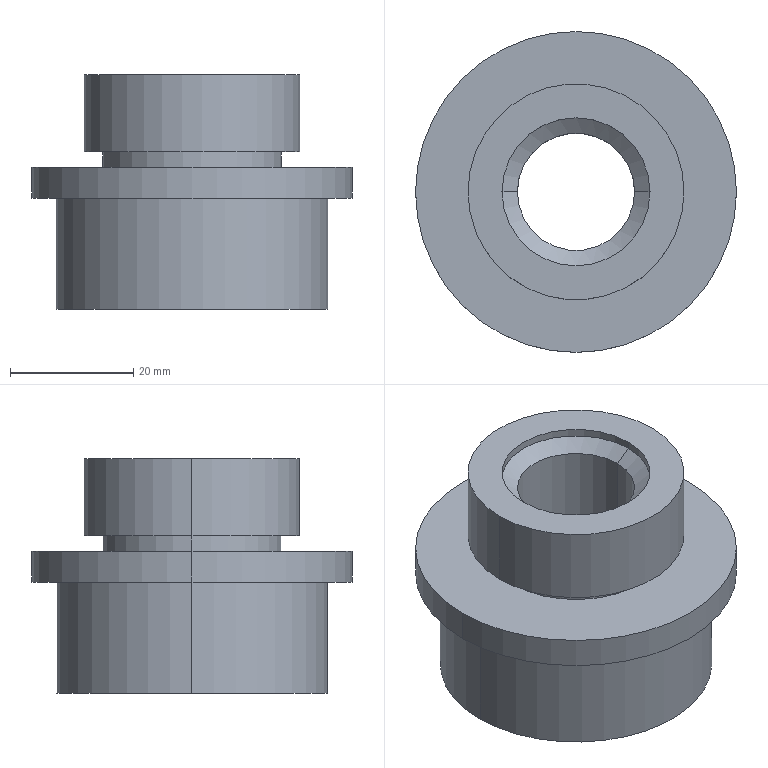Part | SolidWorks | features Revolution 1 | 1 solid | 21 faces | box 52 x 52 x 38 mm | volume 38206 mm3 | cylinder 12 | plane 5 | cone 4 | commonest cylinder face diameters 19 x2 24 x2 29 x2 35 x2 44 x2 52 x2
STEP:
#1=CARTESIAN_POINT('',(17.5,0.,-12.5));
#2=VERTEX_POINT('',#1);
#3=CARTESIAN_POINT('',(-17.5,0.,-12.5));
#4=VERTEX_POINT('',#3);
#5=CARTESIAN_POINT('',(0.,0.,-12.5));
#6=DIRECTION('',(0.,0.,1.));
#7=DIRECTION('',(1.,0.,0.));
#8=AXIS2_PLACEMENT_3D('',#5,#6,#7);
#9=CIRCLE('',#8,17.5);
#10=EDGE_CURVE('',#2,#4,#9,.T.);
#11=ORIENTED_EDGE('',*,*,#10,.T.);
#12=CARTESIAN_POINT('',(-17.5,0.,0.));
#13=VERTEX_POINT('',#12);
#14=CARTESIAN_POINT('',(-17.5,0.,28.492));
#15=DIRECTION('',(0.,0.,1.));
#16=VECTOR('',#15,1000.);
#17=LINE('',#14,#16);
#18=EDGE_CURVE('',#4,#13,#17,.T.);
#19=ORIENTED_EDGE('',*,*,#18,.T.);
#20=CARTESIAN_POINT('',(17.5,0.,0.));
#21=VERTEX_POINT('',#20);
#22=CARTESIAN_POINT('',(0.,0.,0.));
#23=DIRECTION('',(0.,0.,1.));
#24=DIRECTION('',(1.,0.,0.));
#25=AXIS2_PLACEMENT_3D('',#22,#23,#24);
#26=CIRCLE('',#25,17.5);
#27=EDGE_CURVE('',#21,#13,#26,.T.);
#28=ORIENTED_EDGE('',*,*,#27,.F.);
#29=CARTESIAN_POINT('',(17.5,0.,28.492));
#30=DIRECTION('',(0.,0.,1.));
#31=VECTOR('',#30,1000.);
#32=LINE('',#29,#31);
#33=EDGE_CURVE('',#2,#21,#32,.T.);
#34=ORIENTED_EDGE('',*,*,#33,.F.);
#35=EDGE_LOOP('',(#11,#19,#28,#34));
#36=FACE_OUTER_BOUND('',#35,.T.);
#37=CARTESIAN_POINT('',(0.,0.,28.492));
#38=DIRECTION('',(0.,0.,1.));
#39=DIRECTION('',(1.,0.,0.));
#40=AXIS2_PLACEMENT_3D('',#37,#38,#39);
#41=CYLINDRICAL_SURFACE('',#40,17.5);
#42=ADVANCED_FACE('',(#36),#41,.T.);
#43=CARTESIAN_POINT('',(14.5,0.,-15.));
#44=VERTEX_POINT('',#43);
#45=CARTESIAN_POINT('',(-14.5,0.,-15.));
#46=VERTEX_POINT('',#45);
#47=CARTESIAN_POINT('',(0.,0.,-15.));
#48=DIRECTION('',(0.,0.,1.));
#49=DIRECTION('',(1.,0.,0.));
#50=AXIS2_PLACEMENT_3D('',#47,#48,#49);
#51=CIRCLE('',#50,14.5);
#52=EDGE_CURVE('',#44,#46,#51,.T.);
#53=ORIENTED_EDGE('',*,*,#52,.T.);
#54=CARTESIAN_POINT('',(-14.5,0.,-12.5));
#55=VERTEX_POINT('',#54);
#56=CARTESIAN_POINT('',(-14.5,0.,28.492));
#57=DIRECTION('',(0.,0.,1.));
#58=VECTOR('',#57,1000.);
#59=LINE('',#56,#58);
#60=EDGE_CURVE('',#46,#55,#59,.T.);
#61=ORIENTED_EDGE('',*,*,#60,.T.);
#62=CARTESIAN_POINT('',(14.5,0.,-12.5));
#63=VERTEX_POINT('',#62);
#64=CARTESIAN_POINT('',(0.,0.,-12.5));
#65=DIRECTION('',(0.,0.,1.));
#66=DIRECTION('',(1.,0.,0.));
#67=AXIS2_PLACEMENT_3D('',#64,#65,#66);
#68=CIRCLE('',#67,14.5);
#69=EDGE_CURVE('',#63,#55,#68,.T.);
#70=ORIENTED_EDGE('',*,*,#69,.F.);
#71=CARTESIAN_POINT('',(14.5,0.,28.492));
#72=DIRECTION('',(0.,0.,1.));
#73=VECTOR('',#72,1000.);
#74=LINE('',#71,#73);
#75=EDGE_CURVE('',#44,#63,#74,.T.);
#76=ORIENTED_EDGE('',*,*,#75,.F.);
#77=EDGE_LOOP('',(#53,#61,#70,#76));
#78=FACE_OUTER_BOUND('',#77,.T.);
#79=CARTESIAN_POINT('',(0.,0.,28.492));
#80=DIRECTION('',(0.,0.,1.));
#81=DIRECTION('',(1.,0.,0.));
#82=AXIS2_PLACEMENT_3D('',#79,#80,#81);
#83=CYLINDRICAL_SURFACE('',#82,14.5);
#84=ADVANCED_FACE('',(#78),#83,.T.);
#85=CARTESIAN_POINT('',(26.,0.,-20.));
#86=VERTEX_POINT('',#85);
#87=CARTESIAN_POINT('',(-26.,0.,-20.));
#88=VERTEX_POINT('',#87);
#89=CARTESIAN_POINT('',(0.,0.,-20.));
#90=DIRECTION('',(0.,0.,1.));
#91=DIRECTION('',(1.,0.,0.));
#92=AXIS2_PLACEMENT_3D('',#89,#90,#91);
#93=CIRCLE('',#92,26.);
#94=EDGE_CURVE('',#86,#88,#93,.T.);
#95=ORIENTED_EDGE('',*,*,#94,.T.);
#96=CARTESIAN_POINT('',(-26.,0.,-15.));
#97=VERTEX_POINT('',#96);
#98=CARTESIAN_POINT('',(-26.,0.,28.492));
#99=DIRECTION('',(0.,0.,1.));
#100=VECTOR('',#99,1000.);
#101=LINE('',#98,#100);
#102=EDGE_CURVE('',#88,#97,#101,.T.);
#103=ORIENTED_EDGE('',*,*,#102,.T.);
#104=CARTESIAN_POINT('',(26.,0.,-15.));
#105=VERTEX_POINT('',#104);
#106=CARTESIAN_POINT('',(0.,0.,-15.));
#107=DIRECTION('',(0.,0.,1.));
#108=DIRECTION('',(1.,0.,0.));
#109=AXIS2_PLACEMENT_3D('',#106,#107,#108);
#110=CIRCLE('',#109,26.);
#111=EDGE_CURVE('',#105,#97,#110,.T.);
#112=ORIENTED_EDGE('',*,*,#111,.F.);
#113=CARTESIAN_POINT('',(26.,0.,28.492));
#114=DIRECTION('',(0.,0.,1.));
#115=VECTOR('',#114,1000.);
#116=LINE('',#113,#115);
#117=EDGE_CURVE('',#86,#105,#116,.T.);
#118=ORIENTED_EDGE('',*,*,#117,.F.);
#119=EDGE_LOOP('',(#95,#103,#112,#118));
#120=FACE_OUTER_BOUND('',#119,.T.);
#121=CARTESIAN_POINT('',(0.,0.,28.492));
#122=DIRECTION('',(0.,0.,1.));
#123=DIRECTION('',(1.,0.,0.));
#124=AXIS2_PLACEMENT_3D('',#121,#122,#123);
#125=CYLINDRICAL_SURFACE('',#124,26.);
#126=ADVANCED_FACE('',(#120),#125,.T.);
#127=CARTESIAN_POINT('',(22.,0.,-38.));
#128=VERTEX_POINT('',#127);
#129=CARTESIAN_POINT('',(-22.,0.,-38.));
#130=VERTEX_POINT('',#129);
#131=CARTESIAN_POINT('',(0.,0.,-38.));
#132=DIRECTION('',(0.,0.,1.));
#133=DIRECTION('',(1.,0.,0.));
#134=AXIS2_PLACEMENT_3D('',#131,#132,#133);
#135=CIRCLE('',#134,22.);
#136=EDGE_CURVE('',#128,#130,#135,.T.);
#137=ORIENTED_EDGE('',*,*,#136,.T.);
#138=CARTESIAN_POINT('',(-22.,0.,-20.));
#139=VERTEX_POINT('',#138);
#140=CARTESIAN_POINT('',(-22.,0.,28.492));
#141=DIRECTION('',(0.,0.,1.));
#142=VECTOR('',#141,1000.);
#143=LINE('',#140,#142);
#144=EDGE_CURVE('',#130,#139,#143,.T.);
#145=ORIENTED_EDGE('',*,*,#144,.T.);
#146=CARTESIAN_POINT('',(22.,0.,-20.));
#147=VERTEX_POINT('',#146);
#148=CARTESIAN_POINT('',(0.,0.,-20.));
#149=DIRECTION('',(0.,0.,1.));
#150=DIRECTION('',(1.,0.,0.));
#151=AXIS2_PLACEMENT_3D('',#148,#149,#150);
#152=CIRCLE('',#151,22.);
#153=EDGE_CURVE('',#147,#139,#152,.T.);
#154=ORIENTED_EDGE('',*,*,#153,.F.);
#155=CARTESIAN_POINT('',(22.,0.,28.492));
#156=DIRECTION('',(0.,0.,1.));
#157=VECTOR('',#156,1000.);
#158=LINE('',#155,#157);
#159=EDGE_CURVE('',#128,#147,#158,.T.);
#160=ORIENTED_EDGE('',*,*,#159,.F.);
#161=EDGE_LOOP('',(#137,#145,#154,#160));
#162=FACE_OUTER_BOUND('',#161,.T.);
#163=CARTESIAN_POINT('',(0.,0.,28.492));
#164=DIRECTION('',(0.,0.,1.));
#165=DIRECTION('',(1.,0.,0.));
#166=AXIS2_PLACEMENT_3D('',#163,#164,#165);
#167=CYLINDRICAL_SURFACE('',#166,22.);
#168=ADVANCED_FACE('',(#162),#167,.T.);
#169=CARTESIAN_POINT('',(-9.5,0.,-23.));
#170=VERTEX_POINT('',#169);
#171=CARTESIAN_POINT('',(9.5,0.,-23.));
#172=VERTEX_POINT('',#171);
#173=CARTESIAN_POINT('',(0.,0.,-23.));
#174=DIRECTION('',(0.,0.,1.));
#175=DIRECTION('',(1.,0.,0.));
#176=AXIS2_PLACEMENT_3D('',#173,#174,#175);
#177=CIRCLE('',#176,9.5);
#178=EDGE_CURVE('',#170,#172,#177,.T.);
#179=ORIENTED_EDGE('',*,*,#178,.T.);
#180=CARTESIAN_POINT('',(14.,0.,-38.));
#181=VERTEX_POINT('',#180);
#182=CARTESIAN_POINT('',(9.5,0.,-23.));
#183=DIRECTION('',(0.2873,0.,-0.9578));
#184=VECTOR('',#183,1000.);
#185=LINE('',#182,#184);
#186=EDGE_CURVE('',#172,#181,#185,.T.);
#187=ORIENTED_EDGE('',*,*,#186,.T.);
#188=CARTESIAN_POINT('',(-14.,0.,-38.));
#189=VERTEX_POINT('',#188);
#190=CARTESIAN_POINT('',(0.,0.,-38.));
#191=DIRECTION('',(0.,0.,1.));
#192=DIRECTION('',(1.,0.,0.));
#193=AXIS2_PLACEMENT_3D('',#190,#191,#192);
#194=CIRCLE('',#193,14.);
#195=EDGE_CURVE('',#189,#181,#194,.T.);
#196=ORIENTED_EDGE('',*,*,#195,.F.);
#197=CARTESIAN_POINT('',(-9.5,0.,-23.));
#198=DIRECTION('',(-0.2873,0.,-0.9578));
#199=VECTOR('',#198,1000.);
#200=LINE('',#197,#199);
#201=EDGE_CURVE('',#170,#189,#200,.T.);
#202=ORIENTED_EDGE('',*,*,#201,.F.);
#203=EDGE_LOOP('',(#179,#187,#196,#202));
#204=FACE_OUTER_BOUND('',#203,.T.);
#205=CARTESIAN_POINT('',(0.,0.,-23.));
#206=DIRECTION('',(0.,0.,-1.));
#207=DIRECTION('',(-1.,0.,0.));
#208=AXIS2_PLACEMENT_3D('',#205,#206,#207);
#209=CONICAL_SURFACE('',#208,9.5,0.2915);
#210=ADVANCED_FACE('',(#204),#209,.F.);
#211=ORIENTED_EDGE('',*,*,#178,.F.);
#212=CARTESIAN_POINT('',(-9.5,0.,-3.001));
#213=VERTEX_POINT('',#212);
#214=CARTESIAN_POINT('',(-9.5,0.,28.492));
#215=DIRECTION('',(0.,0.,1.));
#216=VECTOR('',#215,1000.);
#217=LINE('',#214,#216);
#218=EDGE_CURVE('',#170,#213,#217,.T.);
#219=ORIENTED_EDGE('',*,*,#218,.T.);
#220=CARTESIAN_POINT('',(9.5,0.,-3.001));
#221=VERTEX_POINT('',#220);
#222=CARTESIAN_POINT('',(0.,0.,-3.001));
#223=DIRECTION('',(0.,0.,1.));
#224=DIRECTION('',(1.,0.,0.));
#225=AXIS2_PLACEMENT_3D('',#222,#223,#224);
#226=CIRCLE('',#225,9.5);
#227=EDGE_CURVE('',#213,#221,#226,.T.);
#228=ORIENTED_EDGE('',*,*,#227,.T.);
#229=CARTESIAN_POINT('',(9.5,0.,28.492));
#230=DIRECTION('',(0.,0.,1.));
#231=VECTOR('',#230,1000.);
#232=LINE('',#229,#231);
#233=EDGE_CURVE('',#172,#221,#232,.T.);
#234=ORIENTED_EDGE('',*,*,#233,.F.);
#235=EDGE_LOOP('',(#211,#219,#228,#234));
#236=FACE_OUTER_BOUND('',#235,.T.);
#237=CARTESIAN_POINT('',(0.,0.,28.492));
#238=DIRECTION('',(0.,0.,1.));
#239=DIRECTION('',(1.,0.,0.));
#240=AXIS2_PLACEMENT_3D('',#237,#238,#239);
#241=CYLINDRICAL_SURFACE('',#240,9.5);
#242=ADVANCED_FACE('',(#236),#241,.F.);
#243=ORIENTED_EDGE('',*,*,#227,.F.);
#244=CARTESIAN_POINT('',(-12.,0.,-1.25));
#245=VERTEX_POINT('',#244);
#246=CARTESIAN_POINT('',(-12.,0.,-1.25));
#247=DIRECTION('',(-0.8192,0.,0.5736));
#248=VECTOR('',#247,1000.);
#249=LINE('',#246,#248);
#250=EDGE_CURVE('',#213,#245,#249,.T.);
#251=ORIENTED_EDGE('',*,*,#250,.T.);
#252=CARTESIAN_POINT('',(12.,0.,-1.25));
#253=VERTEX_POINT('',#252);
#254=CARTESIAN_POINT('',(0.,0.,-1.25));
#255=DIRECTION('',(0.,0.,1.));
#256=DIRECTION('',(1.,0.,0.));
#257=AXIS2_PLACEMENT_3D('',#254,#255,#256);
#258=CIRCLE('',#257,12.);
#259=EDGE_CURVE('',#245,#253,#258,.T.);
#260=ORIENTED_EDGE('',*,*,#259,.T.);
#261=CARTESIAN_POINT('',(12.,0.,-1.25));
#262=DIRECTION('',(0.8192,0.,0.5736));
#263=VECTOR('',#262,1000.);
#264=LINE('',#261,#263);
#265=EDGE_CURVE('',#221,#253,#264,.T.);
#266=ORIENTED_EDGE('',*,*,#265,.F.);
#267=EDGE_LOOP('',(#243,#251,#260,#266));
#268=FACE_OUTER_BOUND('',#267,.T.);
#269=CARTESIAN_POINT('',(0.,0.,-1.25));
#270=DIRECTION('',(0.,0.,1.));
#271=DIRECTION('',(1.,0.,0.));
#272=AXIS2_PLACEMENT_3D('',#269,#270,#271);
#273=CONICAL_SURFACE('',#272,12.,0.9599);
#274=ADVANCED_FACE('',(#268),#273,.F.);
#275=ORIENTED_EDGE('',*,*,#259,.F.);
#276=CARTESIAN_POINT('',(-12.,0.,0.));
#277=VERTEX_POINT('',#276);
#278=CARTESIAN_POINT('',(-12.,0.,28.492));
#279=DIRECTION('',(0.,0.,1.));
#280=VECTOR('',#279,1000.);
#281=LINE('',#278,#280);
#282=EDGE_CURVE('',#245,#277,#281,.T.);
#283=ORIENTED_EDGE('',*,*,#282,.T.);
#284=CARTESIAN_POINT('',(12.,0.,0.));
#285=VERTEX_POINT('',#284);
#286=CARTESIAN_POINT('',(0.,0.,0.));
#287=DIRECTION('',(0.,0.,1.));
#288=DIRECTION('',(1.,0.,0.));
#289=AXIS2_PLACEMENT_3D('',#286,#287,#288);
#290=CIRCLE('',#289,12.);
#291=EDGE_CURVE('',#277,#285,#290,.T.);
#292=ORIENTED_EDGE('',*,*,#291,.T.);
#293=CARTESIAN_POINT('',(12.,0.,28.492));
#294=DIRECTION('',(0.,0.,1.));
#295=VECTOR('',#294,1000.);
#296=LINE('',#293,#295);
#297=EDGE_CURVE('',#253,#285,#296,.T.);
#298=ORIENTED_EDGE('',*,*,#297,.F.);
#299=EDGE_LOOP('',(#275,#283,#292,#298));
#300=FACE_OUTER_BOUND('',#299,.T.);
#301=CARTESIAN_POINT('',(0.,0.,28.492));
#302=DIRECTION('',(0.,0.,1.));
#303=DIRECTION('',(1.,0.,0.));
#304=AXIS2_PLACEMENT_3D('',#301,#302,#303);
#305=CYLINDRICAL_SURFACE('',#304,12.);
#306=ADVANCED_FACE('',(#300),#305,.F.);
#307=ORIENTED_EDGE('',*,*,#282,.F.);
#308=CARTESIAN_POINT('',(0.,0.,-1.25));
#309=DIRECTION('',(0.,0.,1.));
#310=DIRECTION('',(1.,0.,0.));
#311=AXIS2_PLACEMENT_3D('',#308,#309,#310);
#312=CIRCLE('',#311,12.);
#313=EDGE_CURVE('',#253,#245,#312,.T.);
#314=ORIENTED_EDGE('',*,*,#313,.F.);
#315=ORIENTED_EDGE('',*,*,#297,.T.);
#316=CARTESIAN_POINT('',(0.,0.,0.));
#317=DIRECTION('',(0.,0.,1.));
#318=DIRECTION('',(1.,0.,0.));
#319=AXIS2_PLACEMENT_3D('',#316,#317,#318);
#320=CIRCLE('',#319,12.);
#321=EDGE_CURVE('',#285,#277,#320,.T.);
#322=ORIENTED_EDGE('',*,*,#321,.T.);
#323=EDGE_LOOP('',(#307,#314,#315,#322));
#324=FACE_OUTER_BOUND('',#323,.T.);
#325=CARTESIAN_POINT('',(0.,0.,28.492));
#326=DIRECTION('',(0.,0.,1.));
#327=DIRECTION('',(1.,0.,0.));
#328=AXIS2_PLACEMENT_3D('',#325,#326,#327);
#329=CYLINDRICAL_SURFACE('',#328,12.);
#330=ADVANCED_FACE('',(#324),#329,.F.);
#331=ORIENTED_EDGE('',*,*,#250,.F.);
#332=CARTESIAN_POINT('',(0.,0.,-3.001));
#333=DIRECTION('',(0.,0.,1.));
#334=DIRECTION('',(1.,0.,0.));
#335=AXIS2_PLACEMENT_3D('',#332,#333,#334);
#336=CIRCLE('',#335,9.5);
#337=EDGE_CURVE('',#221,#213,#336,.T.);
#338=ORIENTED_EDGE('',*,*,#337,.F.);
#339=ORIENTED_EDGE('',*,*,#265,.T.);
#340=ORIENTED_EDGE('',*,*,#313,.T.);
#341=EDGE_LOOP('',(#331,#338,#339,#340));
#342=FACE_OUTER_BOUND('',#341,.T.);
#343=CARTESIAN_POINT('',(0.,0.,-1.25));
#344=DIRECTION('',(0.,0.,1.));
#345=DIRECTION('',(1.,0.,0.));
#346=AXIS2_PLACEMENT_3D('',#343,#344,#345);
#347=CONICAL_SURFACE('',#346,12.,0.9599);
#348=ADVANCED_FACE('',(#342),#347,.F.);
#349=ORIENTED_EDGE('',*,*,#218,.F.);
#350=CARTESIAN_POINT('',(0.,0.,-23.));
#351=DIRECTION('',(0.,0.,1.));
#352=DIRECTION('',(1.,0.,0.));
#353=AXIS2_PLACEMENT_3D('',#350,#351,#352);
#354=CIRCLE('',#353,9.5);
#355=EDGE_CURVE('',#172,#170,#354,.T.);
#356=ORIENTED_EDGE('',*,*,#355,.F.);
#357=ORIENTED_EDGE('',*,*,#233,.T.);
#358=ORIENTED_EDGE('',*,*,#337,.T.);
#359=EDGE_LOOP('',(#349,#356,#357,#358));
#360=FACE_OUTER_BOUND('',#359,.T.);
#361=CARTESIAN_POINT('',(0.,0.,28.492));
#362=DIRECTION('',(0.,0.,1.));
#363=DIRECTION('',(1.,0.,0.));
#364=AXIS2_PLACEMENT_3D('',#361,#362,#363);
#365=CYLINDRICAL_SURFACE('',#364,9.5);
#366=ADVANCED_FACE('',(#360),#365,.F.);
#367=ORIENTED_EDGE('',*,*,#186,.F.);
#368=ORIENTED_EDGE('',*,*,#355,.T.);
#369=ORIENTED_EDGE('',*,*,#201,.T.);
#370=CARTESIAN_POINT('',(0.,0.,-38.));
#371=DIRECTION('',(0.,0.,1.));
#372=DIRECTION('',(1.,0.,0.));
#373=AXIS2_PLACEMENT_3D('',#370,#371,#372);
#374=CIRCLE('',#373,14.);
#375=EDGE_CURVE('',#181,#189,#374,.T.);
#376=ORIENTED_EDGE('',*,*,#375,.F.);
#377=EDGE_LOOP('',(#367,#368,#369,#376));
#378=FACE_OUTER_BOUND('',#377,.T.);
#379=CARTESIAN_POINT('',(0.,0.,-23.));
#380=DIRECTION('',(0.,0.,-1.));
#381=DIRECTION('',(-1.,0.,0.));
#382=AXIS2_PLACEMENT_3D('',#379,#380,#381);
#383=CONICAL_SURFACE('',#382,9.5,0.2915);
#384=ADVANCED_FACE('',(#378),#383,.F.);
#385=ORIENTED_EDGE('',*,*,#136,.F.);
#386=CARTESIAN_POINT('',(0.,0.,-38.));
#387=DIRECTION('',(0.,0.,1.));
#388=DIRECTION('',(1.,0.,0.));
#389=AXIS2_PLACEMENT_3D('',#386,#387,#388);
#390=CIRCLE('',#389,22.);
#391=EDGE_CURVE('',#130,#128,#390,.T.);
#392=ORIENTED_EDGE('',*,*,#391,.F.);
#393=EDGE_LOOP('',(#385,#392));
#394=FACE_OUTER_BOUND('',#393,.T.);
#395=ORIENTED_EDGE('',*,*,#195,.T.);
#396=ORIENTED_EDGE('',*,*,#375,.T.);
#397=EDGE_LOOP('',(#395,#396));
#398=FACE_BOUND('',#397,.T.);
#399=CARTESIAN_POINT('',(0.,14.,-38.));
#400=DIRECTION('',(0.,0.,1.));
#401=DIRECTION('',(1.,0.,0.));
#402=AXIS2_PLACEMENT_3D('',#399,#400,#401);
#403=PLANE('',#402);
#404=ADVANCED_FACE('',(#394,#398),#403,.F.);
#405=ORIENTED_EDGE('',*,*,#144,.F.);
#406=ORIENTED_EDGE('',*,*,#391,.T.);
#407=ORIENTED_EDGE('',*,*,#159,.T.);
#408=CARTESIAN_POINT('',(0.,0.,-20.));
#409=DIRECTION('',(0.,0.,1.));
#410=DIRECTION('',(1.,0.,0.));
#411=AXIS2_PLACEMENT_3D('',#408,#409,#410);
#412=CIRCLE('',#411,22.);
#413=EDGE_CURVE('',#139,#147,#412,.T.);
#414=ORIENTED_EDGE('',*,*,#413,.F.);
#415=EDGE_LOOP('',(#405,#406,#407,#414));
#416=FACE_OUTER_BOUND('',#415,.T.);
#417=CARTESIAN_POINT('',(0.,0.,28.492));
#418=DIRECTION('',(0.,0.,1.));
#419=DIRECTION('',(1.,0.,0.));
#420=AXIS2_PLACEMENT_3D('',#417,#418,#419);
#421=CYLINDRICAL_SURFACE('',#420,22.);
#422=ADVANCED_FACE('',(#416),#421,.T.);
#423=ORIENTED_EDGE('',*,*,#94,.F.);
#424=CARTESIAN_POINT('',(0.,0.,-20.));
#425=DIRECTION('',(0.,0.,1.));
#426=DIRECTION('',(1.,0.,0.));
#427=AXIS2_PLACEMENT_3D('',#424,#425,#426);
#428=CIRCLE('',#427,26.);
#429=EDGE_CURVE('',#88,#86,#428,.T.);
#430=ORIENTED_EDGE('',*,*,#429,.F.);
#431=EDGE_LOOP('',(#423,#430));
#432=FACE_OUTER_BOUND('',#431,.T.);
#433=ORIENTED_EDGE('',*,*,#153,.T.);
#434=ORIENTED_EDGE('',*,*,#413,.T.);
#435=EDGE_LOOP('',(#433,#434));
#436=FACE_BOUND('',#435,.T.);
#437=CARTESIAN_POINT('',(0.,22.,-20.));
#438=DIRECTION('',(0.,0.,1.));
#439=DIRECTION('',(1.,0.,0.));
#440=AXIS2_PLACEMENT_3D('',#437,#438,#439);
#441=PLANE('',#440);
#442=ADVANCED_FACE('',(#432,#436),#441,.F.);
#443=ORIENTED_EDGE('',*,*,#102,.F.);
#444=ORIENTED_EDGE('',*,*,#429,.T.);
#445=ORIENTED_EDGE('',*,*,#117,.T.);
#446=CARTESIAN_POINT('',(0.,0.,-15.));
#447=DIRECTION('',(0.,0.,1.));
#448=DIRECTION('',(1.,0.,0.));
#449=AXIS2_PLACEMENT_3D('',#446,#447,#448);
#450=CIRCLE('',#449,26.);
#451=EDGE_CURVE('',#97,#105,#450,.T.);
#452=ORIENTED_EDGE('',*,*,#451,.F.);
#453=EDGE_LOOP('',(#443,#444,#445,#452));
#454=FACE_OUTER_BOUND('',#453,.T.);
#455=CARTESIAN_POINT('',(0.,0.,28.492));
#456=DIRECTION('',(0.,0.,1.));
#457=DIRECTION('',(1.,0.,0.));
#458=AXIS2_PLACEMENT_3D('',#455,#456,#457);
#459=CYLINDRICAL_SURFACE('',#458,26.);
#460=ADVANCED_FACE('',(#454),#459,.T.);
#461=ORIENTED_EDGE('',*,*,#52,.F.);
#462=CARTESIAN_POINT('',(0.,0.,-15.));
#463=DIRECTION('',(0.,0.,1.));
#464=DIRECTION('',(1.,0.,0.));
#465=AXIS2_PLACEMENT_3D('',#462,#463,#464);
#466=CIRCLE('',#465,14.5);
#467=EDGE_CURVE('',#46,#44,#466,.T.);
#468=ORIENTED_EDGE('',*,*,#467,.F.);
#469=EDGE_LOOP('',(#461,#468));
#470=FACE_BOUND('',#469,.T.);
#471=ORIENTED_EDGE('',*,*,#111,.T.);
#472=ORIENTED_EDGE('',*,*,#451,.T.);
#473=EDGE_LOOP('',(#471,#472));
#474=FACE_OUTER_BOUND('',#473,.T.);
#475=CARTESIAN_POINT('',(0.,26.,-15.));
#476=DIRECTION('',(0.,0.,-1.));
#477=DIRECTION('',(-1.,0.,0.));
#478=AXIS2_PLACEMENT_3D('',#475,#476,#477);
#479=PLANE('',#478);
#480=ADVANCED_FACE('',(#470,#474),#479,.F.);
#481=ORIENTED_EDGE('',*,*,#60,.F.);
#482=ORIENTED_EDGE('',*,*,#467,.T.);
#483=ORIENTED_EDGE('',*,*,#75,.T.);
#484=CARTESIAN_POINT('',(0.,0.,-12.5));
#485=DIRECTION('',(0.,0.,1.));
#486=DIRECTION('',(1.,0.,0.));
#487=AXIS2_PLACEMENT_3D('',#484,#485,#486);
#488=CIRCLE('',#487,14.5);
#489=EDGE_CURVE('',#55,#63,#488,.T.);
#490=ORIENTED_EDGE('',*,*,#489,.F.);
#491=EDGE_LOOP('',(#481,#482,#483,#490));
#492=FACE_OUTER_BOUND('',#491,.T.);
#493=CARTESIAN_POINT('',(0.,0.,28.492));
#494=DIRECTION('',(0.,0.,1.));
#495=DIRECTION('',(1.,0.,0.));
#496=AXIS2_PLACEMENT_3D('',#493,#494,#495);
#497=CYLINDRICAL_SURFACE('',#496,14.5);
#498=ADVANCED_FACE('',(#492),#497,.T.);
#499=ORIENTED_EDGE('',*,*,#10,.F.);
#500=CARTESIAN_POINT('',(0.,0.,-12.5));
#501=DIRECTION('',(0.,0.,1.));
#502=DIRECTION('',(1.,0.,0.));
#503=AXIS2_PLACEMENT_3D('',#500,#501,#502);
#504=CIRCLE('',#503,17.5);
#505=EDGE_CURVE('',#4,#2,#504,.T.);
#506=ORIENTED_EDGE('',*,*,#505,.F.);
#507=EDGE_LOOP('',(#499,#506));
#508=FACE_OUTER_BOUND('',#507,.T.);
#509=ORIENTED_EDGE('',*,*,#69,.T.);
#510=ORIENTED_EDGE('',*,*,#489,.T.);
#511=EDGE_LOOP('',(#509,#510));
#512=FACE_BOUND('',#511,.T.);
#513=CARTESIAN_POINT('',(0.,14.5,-12.5));
#514=DIRECTION('',(0.,0.,1.));
#515=DIRECTION('',(1.,0.,0.));
#516=AXIS2_PLACEMENT_3D('',#513,#514,#515);
#517=PLANE('',#516);
#518=ADVANCED_FACE('',(#508,#512),#517,.F.);
#519=ORIENTED_EDGE('',*,*,#18,.F.);
#520=ORIENTED_EDGE('',*,*,#505,.T.);
#521=ORIENTED_EDGE('',*,*,#33,.T.);
#522=CARTESIAN_POINT('',(0.,0.,0.));
#523=DIRECTION('',(0.,0.,1.));
#524=DIRECTION('',(1.,0.,0.));
#525=AXIS2_PLACEMENT_3D('',#522,#523,#524);
#526=CIRCLE('',#525,17.5);
#527=EDGE_CURVE('',#13,#21,#526,.T.);
#528=ORIENTED_EDGE('',*,*,#527,.F.);
#529=EDGE_LOOP('',(#519,#520,#521,#528));
#530=FACE_OUTER_BOUND('',#529,.T.);
#531=CARTESIAN_POINT('',(0.,0.,28.492));
#532=DIRECTION('',(0.,0.,1.));
#533=DIRECTION('',(1.,0.,0.));
#534=AXIS2_PLACEMENT_3D('',#531,#532,#533);
#535=CYLINDRICAL_SURFACE('',#534,17.5);
#536=ADVANCED_FACE('',(#530),#535,.T.);
#537=ORIENTED_EDGE('',*,*,#321,.F.);
#538=ORIENTED_EDGE('',*,*,#291,.F.);
#539=EDGE_LOOP('',(#537,#538));
#540=FACE_BOUND('',#539,.T.);
#541=ORIENTED_EDGE('',*,*,#27,.T.);
#542=ORIENTED_EDGE('',*,*,#527,.T.);
#543=EDGE_LOOP('',(#541,#542));
#544=FACE_OUTER_BOUND('',#543,.T.);
#545=CARTESIAN_POINT('',(0.,17.5,0.));
#546=DIRECTION('',(0.,0.,-1.));
#547=DIRECTION('',(-1.,0.,0.));
#548=AXIS2_PLACEMENT_3D('',#545,#546,#547);
#549=PLANE('',#548);
#550=ADVANCED_FACE('',(#540,#544),#549,.F.);
#551=CLOSED_SHELL('',(#42,#84,#126,#168,#210,#242,#274,#306,#330,#348,#366,#384,#404,#422,#442,#460,#480,#498,#518,#536,#550));
#552=MANIFOLD_SOLID_BREP('',#551);
#553=CARTESIAN_POINT('',(0.,0.,0.));
#554=DIRECTION('',(0.,0.,1.));
#555=DIRECTION('',(1.,0.,0.));
#556=AXIS2_PLACEMENT_3D('',#553,#554,#555);
#557=(LENGTH_UNIT()NAMED_UNIT(*)SI_UNIT(.MILLI.,.METRE.));
#558=UNCERTAINTY_MEASURE_WITH_UNIT(LENGTH_MEASURE(0.00001),#557,'','');
#559=(NAMED_UNIT(*)PLANE_ANGLE_UNIT()SI_UNIT($,.RADIAN.));
#560=(NAMED_UNIT(*)SI_UNIT($,.STERADIAN.)SOLID_ANGLE_UNIT());
#561=(GEOMETRIC_REPRESENTATION_CONTEXT(3)GLOBAL_UNCERTAINTY_ASSIGNED_CONTEXT((#558))GLOBAL_UNIT_ASSIGNED_CONTEXT((#557,#559,#560))REPRESENTATION_CONTEXT('',''));
#562=ADVANCED_BREP_SHAPE_REPRESENTATION('',(#552,#556),#561);